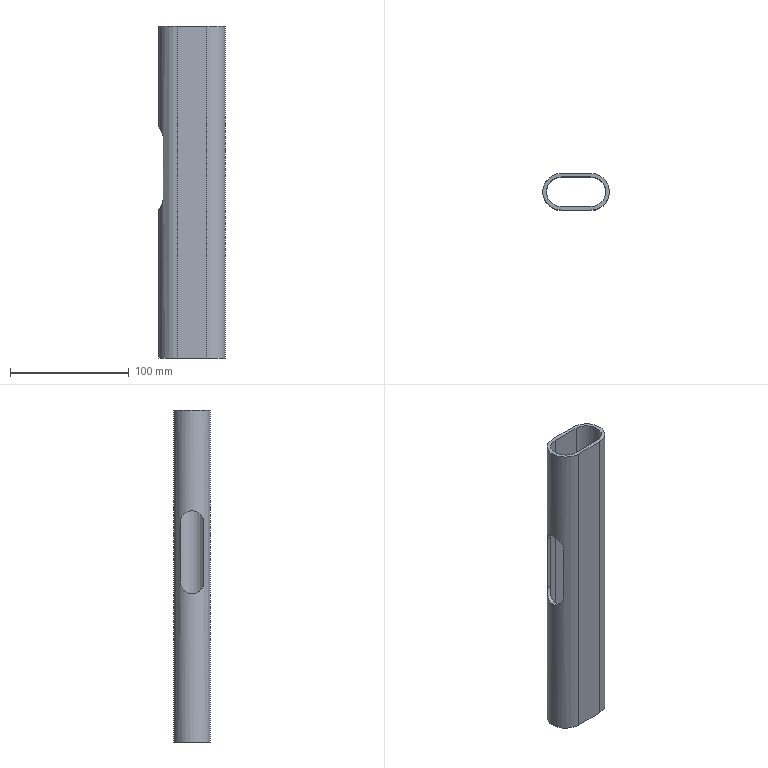Part | STEP file | 5091202W | 1 solid | 14 faces | box 56 x 31 x 280 mm | volume 111520 mm3 | plane 8 | cylinder 6 | commonest cylinder face diameters 20 x2 25 x2 31 x2